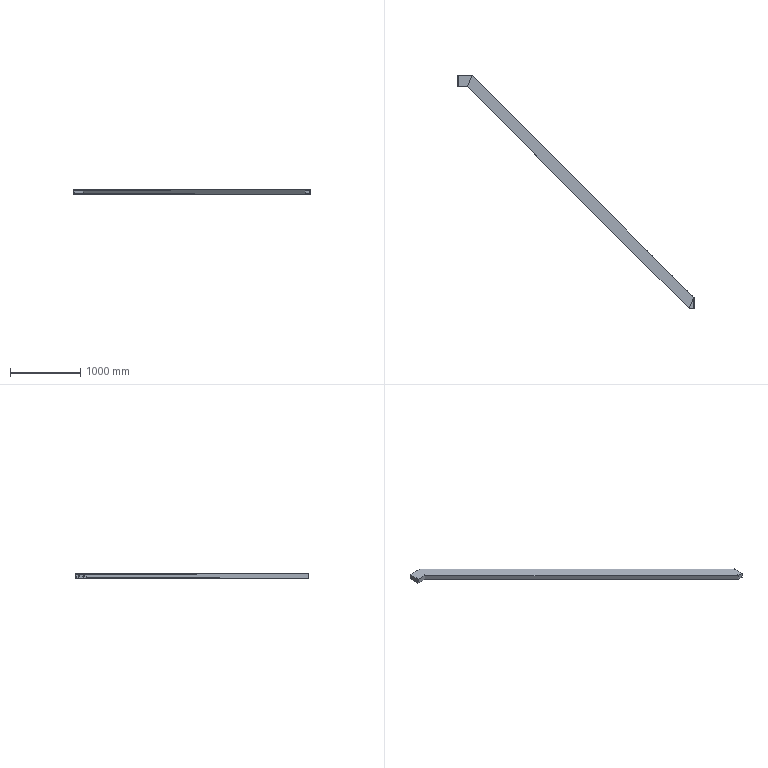Part | STEP file | PN_0045 second-floor stair beam [16a_Default<As Machined> | 5 solids | 71 faces | box 3362 x 3310 x 63 mm | volume 10264966 mm3 | plane 41 | cylinder 30 | commonest cylinder face diameters 6.8 x12 10 x6 20 x6 18 x4 25 x2